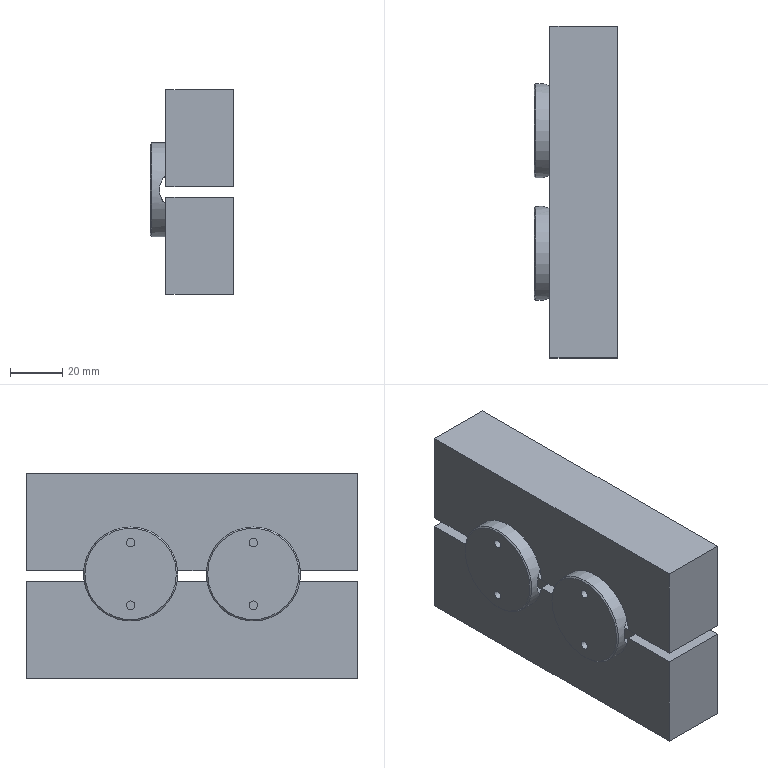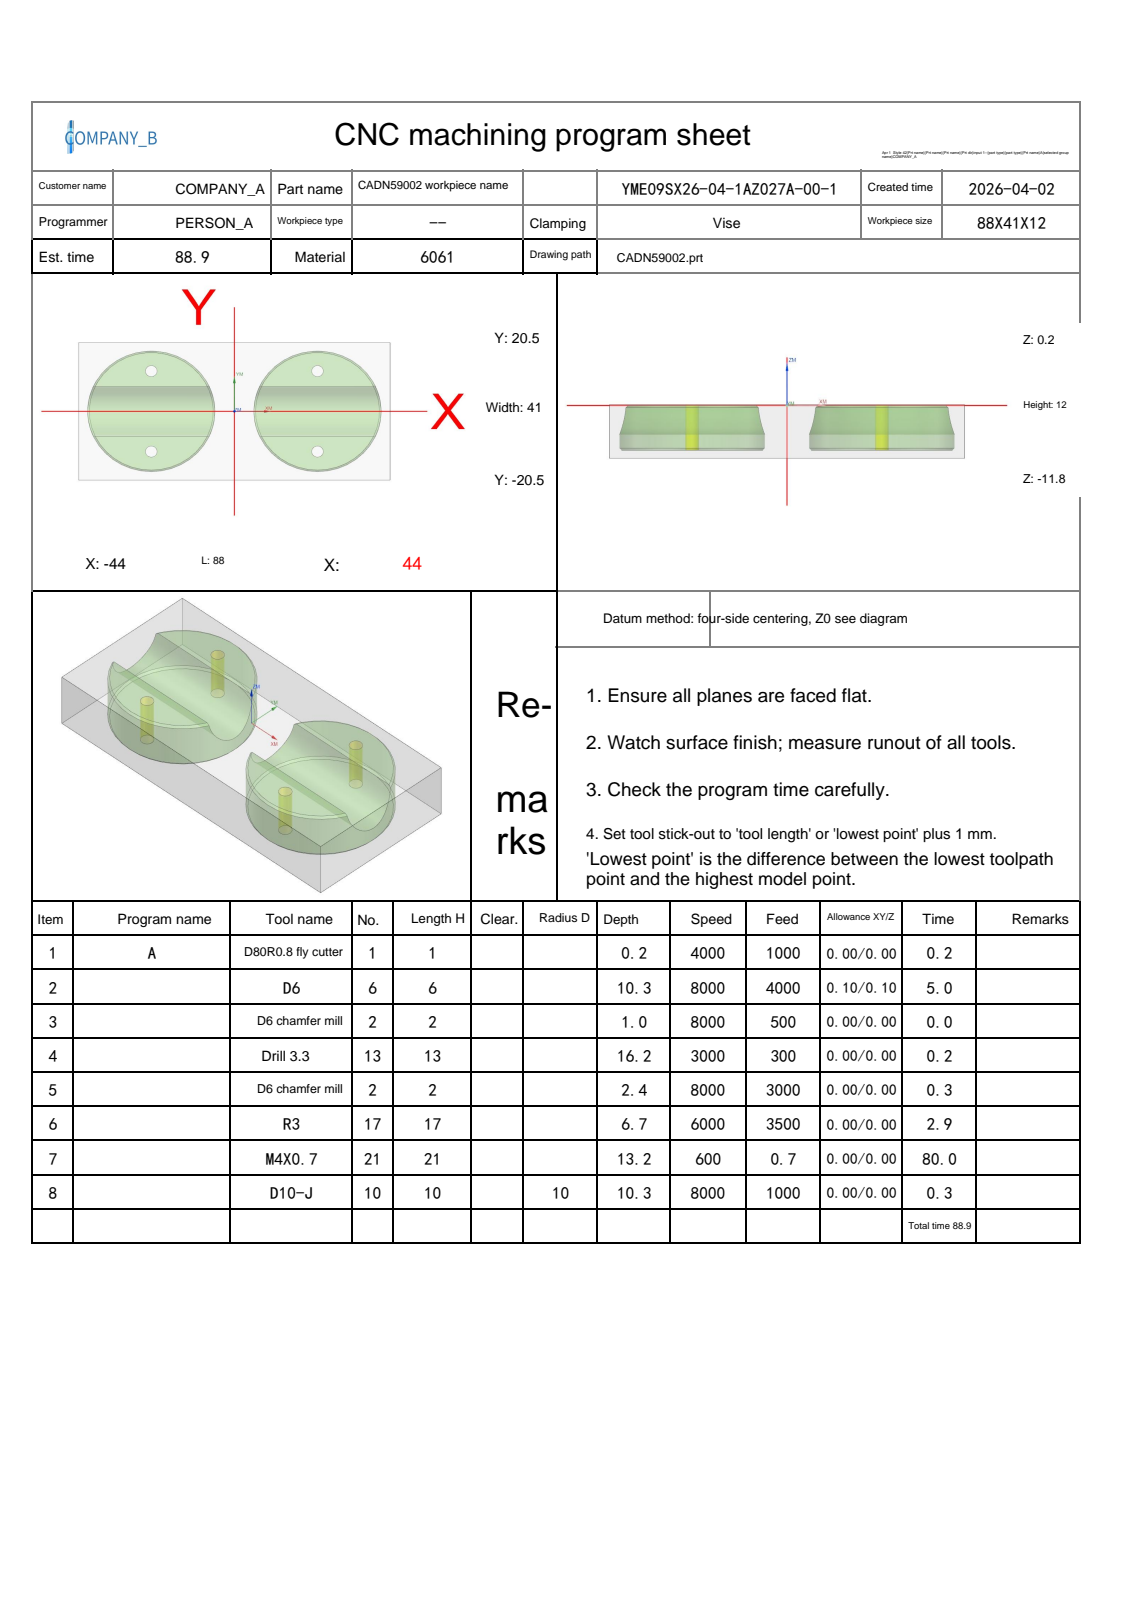NC program | NX | posted by the shop | part box 32 x 127 x 78.432 mm
Lines 34 to 1083 of 8369:
N2 T06 M06
(D6  D=6. R=0. H=06 ce=0.10 di=0.10)
G00 G90 G54 X-51.2 Y-4.2 M03 S8000
G43 H06 Z10.2
M08
Z.719
G01 Z-.481 F4000.
X-48.5
G03 X-44.3 Y0.0 I0.0 J4.2
G01 Y20.5
G02 X-44. Y20.8 I.3 J0.0
G01 X-39.372
G02 X-38.772 Y20.2 I0.0 J-.6
G01 X-38.78 Y20.1
X-39.137 Y17.99
G03 X-39.174 Y17.554 I2.581 J-.436
X-38.848 Y16.29 I2.618 J0.0
G02 X-38.774 Y16. I-.525 J-.29
X-38.95 Y15.575 I-.6 J0.0
G01 X-39.075 Y15.45
G02 X-39.5 Y15.274 I-.425 J.424
X-40.1 Y15.872 I0.0 J.6
G01 Y16.001
G02 X-39.83 Y16.501 I.6 J-.001
G03 X-39.56 Y17.002 I-.33 J.501
G01 X-39.565 Y17.081
X-39.967 Y20.121
X-39.972 Y20.2
G02 X-39.372 Y20.8 I.6 J0.0
G01 X-30.474
G02 X-23.5 Y21.938 I6.974 J-20.8
X-16.526 Y20.8 I0.0 J-21.938
G01 X16.526
G02 X23.5 Y21.938 I6.974 J-20.8
X30.474 Y20.8 I0.0 J-21.938
G01 X44.
G02 X44.3 Y20.5 I0.0 J-.3
G01 Y15.872
G02 X43.7 Y15.272 I-.6 J0.0
G01 X43.6 Y15.28
X41.49 Y15.637
G03 X41.054 Y15.674 I-.436 J-2.581
X39.79 Y15.348 I0.0 J-2.618
G02 X39.5 Y15.274 I-.29 J.525
X39.075 Y15.45 I0.0 J.6
G01 X38.95 Y15.575
G02 X38.774 Y16. I.424 J.425
X39.372 Y16.6 I.6 J0.0
G01 X39.501
G02 X40.001 Y16.33 I-.001 J-.6
G03 X40.502 Y16.06 I.501 J.33
G01 X40.581 Y16.065
X43.621 Y16.467
X43.7 Y16.472
G02 X44.3 Y15.872 I0.0 J-.6
G01 Y-20.5
G02 X44. Y-20.8 I-.3 J0.0
G01 X39.372
G02 X38.772 Y-20.2 I0.0 J.6
G01 X38.78 Y-20.1
X39.137 Y-17.99
G03 X39.174 Y-17.554 I-2.581 J.436
X38.848 Y-16.29 I-2.618 J0.0
G02 X38.774 Y-16. I.525 J.29
X38.95 Y-15.575 I.6 J0.0
G01 X39.075 Y-15.45
G02 X39.5 Y-15.274 I.425 J-.424
X40.1 Y-15.872 I0.0 J-.6
G01 Y-16.001
G02 X39.83 Y-16.501 I-.6 J.001
G03 X39.56 Y-17.002 I.33 J-.501
G01 X39.565 Y-17.081
X39.967 Y-20.121
X39.972 Y-20.2
G02 X39.372 Y-20.8 I-.6 J0.0
G01 X30.474
G02 X23.5 Y-21.938 I-6.974 J20.8
X16.526 Y-20.8 I0.0 J21.938
G01 X-16.526
G02 X-23.5 Y-21.938 I-6.974 J20.8
X-30.474 Y-20.8 I0.0 J21.938
G01 X-44.
G02 X-44.3 Y-20.5 I0.0 J.3
G01 Y-15.872
G02 X-43.7 Y-15.272 I.6 J0.0
G01 X-43.6 Y-15.28
X-41.49 Y-15.637
G03 X-41.054 Y-15.674 I.436 J2.581
X-39.79 Y-15.348 I0.0 J2.618
G02 X-39.5 Y-15.274 I.29 J-.525
X-39.075 Y-15.45 I0.0 J-.6
G01 X-38.95 Y-15.575
G02 X-38.774 Y-16. I-.424 J-.425
X-39.372 Y-16.6 I-.6 J0.0
G01 X-39.501
G02 X-40.001 Y-16.33 I.001 J.6
G03 X-40.502 Y-16.06 I-.501 J-.33
G01 X-40.581 Y-16.065
X-43.621 Y-16.467
X-43.7 Y-16.472
G02 X-44.3 Y-15.872 I0.0 J.6
G01 Y3.
G02 X-43.7 Y3.6 I.6 J0.0
G01 X-43.573 Y3.586
X-40.589 Y2.94
X-40.463 Y2.927
G03 X-39.982 Y3.168 I0.0 J.6
G02 X-39.501 Y3.41 I.482 J-.358
G01 X-7.068
G03 X-4.389 Y4.463 I-.001 J3.939
G02 X-4.185 Y4.587 I.408 J-.44
G01 X-1.896 Y5.416
G03 X-1.5 Y5.981 I-.204 J.564
G01 Y10.182
G02 X0.0 Y11.682 I1.5 J0.0
X1.5 Y10.182 I0.0 J-1.5
G01 Y4.372
G02 X0.0 Y2.872 I-1.5 J0.0
X-.984 Y3.24 I0.0 J1.5
G01 X-1.093 Y3.365
X-3.075 Y6.414
G02 X-3.171 Y6.741 I.503 J.327
G01 X-3.166 Y6.821
G03 X-3.13 Y7.349 I-3.903 J.528
X-3.474 Y8.958 I-3.939 J0.0
X-7.838 Y15.362 I-20.026 J-8.958
X-8.171 Y15.502 I-.334 J-.327
G01 X-8.33 Y15.474
X-8.55 Y15.395
G03 X-8.716 Y15.158 I.086 J-.237
G01 X-8.642 Y14.979
G02 X-4.241 Y8.615 I-14.858 J-14.979
X-3.97 Y7.349 I-2.828 J-1.266
X-7.068 Y4.25 I-3.099 J0.0
G01 X-39.932
G02 X-43.026 Y7.355 I.01 J3.104
X-42.751 Y8.634 I3.104 J0.0
X-23.5 Y21.098 I19.251 J-8.634
X-8.642 Y14.979 I0.0 J-21.098
G01 X-8.464 Y14.906
G03 X-8.226 Y15.074 I0.0 J.252
G01 X-8.095 Y15.448
X-8.081 Y15.528
X-8.123 Y15.663
G02 X-8.226 Y16. I.496 J.337
X-7.628 Y16.6 I.6 J0.0
G01 X7.628
G02 X8.226 Y16. I-.001 J-.6
X8.05 Y15.575 I-.6 J0.0
G03 X4.882 Y11.605 I15.45 J-15.575
G02 X4.373 Y11.322 I-.509 J.318
G01 X4.294 Y11.328
X.645 Y11.814
X.485 Y11.825
G03 X.08 Y11.755 I0.0 J-1.216
G01 X0.0 Y11.742
G02 X-.213 Y11.872 I0.0 J.24
G01 X-.305 Y12.05
X-.332 Y12.16
G02 X-.093 Y12.4 I.24 J0.0
G01 X.093
G02 X.331 Y12.181 I-.001 J-.24
G03 X.464 Y11.869 I.544 J.048
G01 X3.117 Y8.847
G02 X3.266 Y8.451 I-.451 J-.396
G01 X3.248 Y8.306
G03 X3.13 Y7.349 I3.821 J-.957
X7.068 Y3.41 I3.939 J0.0
G01 X39.206
G03 X39.628 Y3.677 I0.0 J.467
G01 X39.729 Y3.89
X39.753 Y3.998
G03 X39.501 Y4.25 I-.252 J0.0
G01 X7.068
G02 X3.97 Y7.349 I.001 J3.099
X4.241 Y8.615 I3.099 J0.0
X23.5 Y21.098 I19.259 J-8.615
X42.751 Y8.634 I0.0 J-21.098
X43.029 Y7.349 I-2.821 J-1.285
X39.929 Y4.249 I-3.1 J0.0
G01 X39.846 Y4.25
X39.501
G03 X39.249 Y3.998 I0.0 J-.252
G01 X39.274 Y3.89
X39.444 Y3.532
G03 X39.615 Y3.399 I.217 J.103
G02 X40.1 Y2.812 I-.115 J-.589
G01 Y.497
X40.088 Y.467
X40.059 Y.438
X40.039 Y.392
G02 X38.56 Y-1.071 I-1.5 J.037
G01 X4.521 Y-1.519
X4.501
G02 X3.001 Y-.019 I0.0 J1.5
X4.481 Y1.481 I1.5 J0.0
G01 X38.52 Y1.929
X38.54
G02 X40.038 Y.496 I0.0 J-1.5
G01 X40.051 Y.467
X40.08 Y.439
X40.1 Y.39
Y-2.812
G02 X39.501 Y-3.41 I-.6 J.001
G01 X7.068
G03 X3.13 Y-7.349 I.001 J-3.939
X3.166 Y-7.878 I3.939 J0.0
G01 X3.172 Y-7.958
G02 X3.032 Y-8.342 I-.6 J0.0
G01 X1.626 Y-10.03
G03 X1.491 Y-10.348 I.461 J-.384
G02 X0.0 Y-11.682 I-1.491 J.166
X-1.5 Y-10.182 I0.0 J1.5
G01 Y-4.372
G02 X0.0 Y-2.872 I1.5 J0.0
X1.5 Y-4.372 I0.0 J-1.5
G01 Y-8.648
G03 X1.846 Y-9.191 I.6 J0.0
G01 X3.921 Y-10.162
G02 X4.194 Y-10.42 I-.254 J-.543
G03 X7.838 Y-15.362 I19.306 J10.42
X8.171 Y-15.502 I.334 J.327
G01 X8.33 Y-15.474
X8.55 Y-15.395
G03 X8.716 Y-15.158 I-.086 J.237
G01 X8.642 Y-14.979
G02 X4.241 Y-8.615 I14.858 J14.979
X3.97 Y-7.349 I2.828 J1.266
X7.068 Y-4.25 I3.099 J0.0
G01 X39.932
G02 X43.026 Y-7.355 I-.01 J-3.104
X42.751 Y-8.634 I-3.104 J0.0
X23.5 Y-21.098 I-19.251 J8.634
X8.642 Y-14.979 I0.0 J21.098
G01 X8.464 Y-14.906
G03 X8.226 Y-15.074 I0.0 J-.252
G01 X8.095 Y-15.448
X8.081 Y-15.528
X8.123 Y-15.663
G02 X8.226 Y-16. I-.496 J-.337
X7.628 Y-16.6 I-.6 J0.0
G01 X-7.628
G02 X-8.226 Y-16. I.001 J.6
X-8.05 Y-15.575 I.6 J0.0
G03 X-4.882 Y-11.605 I-15.45 J15.575
G02 X-4.373 Y-11.322 I.509 J-.318
G01 X-4.294 Y-11.328
X-.645 Y-11.814
X-.485 Y-11.825
G03 X-.08 Y-11.755 I0.0 J1.216
G01 X0.0 Y-11.742
G02 X.213 Y-11.872 I0.0 J-.24
G01 X.305 Y-12.05
X.332 Y-12.16
G02 X.093 Y-12.4 I-.24 J0.0
G01 X-.093
G02 X-.331 Y-12.181 I.001 J.24
G03 X-.464 Y-11.869 I-.544 J-.048
G01 X-3.117 Y-8.847
G02 X-3.266 Y-8.451 I.451 J.396
G01 X-3.248 Y-8.306
G03 X-3.13 Y-7.349 I-3.821 J.957
X-3.722 Y-5.274 I-3.939 J0.0
G02 X-3.812 Y-4.958 I.51 J.316
G01 X-3.792 Y-4.806
X-2.752 Y-.828
X-2.732 Y-.676
G03 X-2.836 Y-.338 I-.6 J0.0
G02 X-2.941 Y0.0 I.496 J.338
X-2.667 Y.504 I.6 J0.0
G03 X-.484 Y2.566 I-4.402 J6.845
G02 X0.0 Y2.812 I.484 J-.354
X.484 Y2.566 I0.0 J-.6
G03 X2.667 Y.504 I6.585 J4.783
G02 X2.941 Y0.0 I-.326 J-.504
X2.667 Y-.504 I-.6 J0.0
G03 X.484 Y-2.566 I4.402 J-6.845
G02 X0.0 Y-2.812 I-.484 J.354
X-.484 Y-2.566 I0.0 J.6
G03 X-1.19 Y-1.721 I-6.585 J-4.783
X-1.623 Y-1.536 I-.433 J-.415
X-1.858 Y-1.584 I0.0 J-.6
G01 X-6.161 Y-3.413
G02 X-6.395 Y-3.461 I-.234 J.552
G01 X-6.484 Y-3.454
G03 X-7.068 Y-3.41 I-.585 J-3.895
G01 X-39.206
G03 X-39.628 Y-3.677 I0.0 J-.467
G01 X-39.729 Y-3.89
X-39.753 Y-3.998
G03 X-39.501 Y-4.25 I.252 J0.0
G01 X-7.068
G02 X-3.97 Y-7.349 I-.001 J-3.099
X-4.241 Y-8.615 I-3.099 J0.0
X-23.5 Y-21.098 I-19.259 J8.615
X-42.751 Y-8.634 I0.0 J21.098
X-43.029 Y-7.349 I2.821 J1.285
X-39.929 Y-4.249 I3.1 J0.0
G01 X-39.846 Y-4.25
X-39.501
G03 X-39.249 Y-3.998 I0.0 J.252
G01 X-39.274 Y-3.89
X-39.444 Y-3.532
G03 X-39.615 Y-3.399 I-.217 J-.103
G02 X-40.1 Y-2.812 I.115 J.589
G01 Y-.497
X-40.088 Y-.467
X-40.059 Y-.438
X-40.039 Y-.392
G02 X-38.56 Y1.071 I1.5 J-.037
G01 X-4.521 Y1.519
X-4.501
G02 X-3.001 Y.019 I0.0 J-1.5
X-4.481 Y-1.481 I-1.5 J0.0
G01 X-38.52 Y-1.929
X-38.54
G02 X-40.038 Y-.496 I0.0 J1.5
G01 X-40.051 Y-.467
X-40.08 Y-.439
X-40.1 Y-.39
Y0.0
Y2.834
G02 X-39.886 Y3.27 I.6 J-.024
G01 X-40.69 Y2.595 Z.569
G00 Z3.
G01 X-51.2 Y-4.2 F6000.
G00 Z.238
G01 Z-.962 F4000.
X-48.5
G03 X-44.3 Y0.0 I0.0 J4.2
G01 Y20.5
G02 X-44. Y20.8 I.3 J0.0
G01 X-39.375
G02 X-38.775 Y20.2 I0.0 J-.6
G01 X-38.783 Y20.1
X-39.14 Y17.988
G03 X-39.176 Y17.553 I2.577 J-.435
X-38.851 Y16.29 I2.614 J0.0
G02 X-38.776 Y16. I-.525 J-.29
X-38.952 Y15.575 I-.6 J0.0
G01 X-39.075 Y15.452
G02 X-39.5 Y15.276 I-.425 J.424
X-40.1 Y15.875 I0.0 J.6
G01 Y16.002
G02 X-39.83 Y16.501 I.6 J-.002
G03 X-39.56 Y17.002 I-.33 J.501
G01 X-39.565 Y17.081
X-39.969 Y20.121
X-39.975 Y20.2
G02 X-39.375 Y20.8 I.6 J0.0
G01 X-30.48
G02 X-23.5 Y21.94 I6.98 J-20.8
X-16.52 Y20.8 I0.0 J-21.94
G01 X16.52
G02 X23.5 Y21.94 I6.98 J-20.8
X30.48 Y20.8 I0.0 J-21.94
G01 X44.
G02 X44.3 Y20.5 I0.0 J-.3
G01 Y15.875
G02 X43.7 Y15.275 I-.6 J0.0
G01 X43.6 Y15.283
X41.488 Y15.64
G03 X41.053 Y15.676 I-.435 J-2.577
X39.79 Y15.351 I0.0 J-2.614
G02 X39.5 Y15.276 I-.29 J.525
X39.075 Y15.452 I0.0 J.6
G01 X38.952 Y15.575
G02 X38.776 Y16. I.424 J.425
X39.375 Y16.6 I.6 J0.0
G01 X39.502
G02 X40.001 Y16.33 I-.002 J-.6
G03 X40.502 Y16.06 I.501 J.33
G01 X40.581 Y16.065
X43.621 Y16.469
X43.7 Y16.475
G02 X44.3 Y15.875 I0.0 J-.6
G01 Y-20.5
G02 X44. Y-20.8 I-.3 J0.0
G01 X39.375
G02 X38.775 Y-20.2 I0.0 J.6
G01 X38.783 Y-20.1
X39.14 Y-17.988
G03 X39.176 Y-17.553 I-2.577 J.435
X38.851 Y-16.29 I-2.614 J0.0
G02 X38.776 Y-16. I.525 J.29
X38.952 Y-15.575 I.6 J0.0
G01 X39.075 Y-15.452
G02 X39.5 Y-15.276 I.425 J-.424
X40.1 Y-15.875 I0.0 J-.6
G01 Y-16.002
G02 X39.83 Y-16.501 I-.6 J.002
G03 X39.56 Y-17.002 I.33 J-.501
G01 X39.565 Y-17.081
X39.969 Y-20.121
X39.975 Y-20.2
G02 X39.375 Y-20.8 I-.6 J0.0
G01 X30.48
G02 X23.5 Y-21.94 I-6.98 J20.8
X16.52 Y-20.8 I0.0 J21.94
G01 X-16.52
G02 X-23.5 Y-21.94 I-6.98 J20.8
X-30.48 Y-20.8 I0.0 J21.94
G01 X-44.
G02 X-44.3 Y-20.5 I0.0 J.3
G01 Y-15.875
G02 X-43.7 Y-15.275 I.6 J0.0
G01 X-43.6 Y-15.283
X-41.488 Y-15.64
G03 X-41.053 Y-15.676 I.435 J2.577
X-39.79 Y-15.351 I0.0 J2.614
G02 X-39.5 Y-15.276 I.29 J-.525
X-39.075 Y-15.452 I0.0 J-.6
G01 X-38.952 Y-15.575
G02 X-38.776 Y-16. I-.424 J-.425
X-39.375 Y-16.6 I-.6 J0.0
G01 X-39.502
G02 X-40.001 Y-16.33 I.002 J.6
G03 X-40.502 Y-16.06 I-.501 J-.33
G01 X-40.581 Y-16.065
X-43.621 Y-16.469
X-43.7 Y-16.475
G02 X-44.3 Y-15.875 I0.0 J.6
G01 Y3.
G02 X-43.7 Y3.6 I.6 J0.0
G01 X-43.557 Y3.583
X-40.587 Y2.853
X-40.444 Y2.836
G03 X-39.972 Y3.065 I0.0 J.6
G02 X-39.502 Y3.295 I.472 J-.37
G01 X-7.08
X-7.009
G03 X-3.075 Y7.229 I0.0 J3.934
X-3.412 Y8.823 I-3.934 J0.0
X-7.835 Y15.362 I-20.088 J-8.823
X-8.169 Y15.502 I-.334 J-.327
G01 X-8.328 Y15.474
X-8.547 Y15.395
G03 X-8.714 Y15.158 I.086 J-.237
G01 X-8.639 Y14.979
G02 X-4.181 Y8.483 I-14.861 J-14.979
X-3.915 Y7.229 I-2.828 J-1.255
X-7.009 Y4.135 I-3.094 J0.0
G01 X-7.072
X-39.984
X-40.003
G02 X-43.089 Y7.221 I0.0 J3.086
X-42.819 Y8.483 I3.086 J0.0
X-23.5 Y21.1 I19.319 J-8.483
X-8.639 Y14.979 I0.0 J-21.1
G01 X-8.462 Y14.906
G03 X-8.224 Y15.074 I0.0 J.252
G01 X-8.092 Y15.448
X-8.079 Y15.528
X-8.12 Y15.663
G02 X-8.224 Y16. I.496 J.337
X-7.625 Y16.6 I.6 J0.0
G01 X7.625
G02 X8.224 Y16. I-.002 J-.6
X8.048 Y15.575 I-.6 J0.0
G03 X4.882 Y11.608 I15.452 J-15.575
G02 X4.373 Y11.326 I-.509 J.318
G01 X4.294 Y11.331
X.644 Y11.818
X.484 Y11.829
G03 X.08 Y11.759 I0.0 J-1.211
G01 X0.0 Y11.746
G02 X-.213 Y11.876 I0.0 J.24
G01 X-.303 Y12.05
X-.33 Y12.16
G02 X-.091 Y12.4 I.24 J0.0
G01 X.091
G02 X.329 Y12.181 I-.001 J-.24
G03 X.461 Y11.87 I.541 J.047
G01 X3.098 Y8.864
G02 X3.247 Y8.469 I-.451 J-.395
G01 X3.224 Y8.305
G03 X3.074 Y7.23 I3.786 J-1.075
X3.116 Y6.662 I3.935 J0.0
G01 X3.122 Y6.575
G02 X3.005 Y6.219 I-.6 J0.0
G01 X1.606 Y4.321
G03 X1.492 Y4.026 I.483 J-.356
G02 X0.0 Y2.677 I-1.492 J.151
X-1.5 Y4.177 I0.0 J1.5
G01 Y10.185
G02 X0.0 Y11.686 I1.5 J0.0
X1.5 Y10.186 I0.0 J-1.5
G01 Y5.785
G03 X1.903 Y5.219 I.6 J0.0
G01 X4.167 Y4.431
G02 X4.371 Y4.31 I-.197 J-.567
G03 X7.01 Y3.295 I2.638 J2.92
G01 X7.08
X39.206
G03 X39.628 Y3.562 I0.0 J.467
G01 X39.729 Y3.775
X39.754 Y3.883
G03 X39.502 Y4.135 I-.252 J0.0
G01 X7.072
X7.01
G02 X3.914 Y7.23 I0.0 J3.095
X4.209 Y8.549 I3.095 J0.0
X23.5 Y21.1 I19.291 J-8.549
X42.819 Y8.483 I0.0 J-21.1
X43.089 Y7.221 I-2.816 J-1.262
X40.003 Y4.135 I-3.086 J0.0
G01 X39.985
X39.502
G03 X39.25 Y3.883 I0.0 J-.252
G01 X39.274 Y3.775
X39.444 Y3.417
G03 X39.615 Y3.284 I.217 J.103
G02 X40.1 Y2.697 I-.115 J-.589
G01 Y.371
X40.088 Y.34
X40.059 Y.312
X40.039 Y.266
G02 X38.554 Y-1.191 I-1.499 J.042
G01 X4.281 Y-1.514
X4.267
G02 X2.767 Y-.014 I0.0 J1.5
X4.253 Y1.486 I1.5 J0.0
G01 X38.526 Y1.809
X38.54
G02 X40.039 Y.37 I0.0 J-1.5
G01 X40.051 Y.341
X40.08 Y.313
X40.1 Y.264
Y-2.697
G02 X39.502 Y-3.295 I-.6 J.002
G01 X7.016
X7.009
G03 X3.074 Y-7.23 I0.0 J-3.935
X3.445 Y-8.898 I3.935 J0.0
X7.835 Y-15.362 I20.055 J8.898
X8.169 Y-15.502 I.334 J.327
G01 X8.328 Y-15.474
X8.547 Y-15.395
G03 X8.714 Y-15.158 I-.086 J.237
G01 X8.639 Y-14.979
G02 X4.209 Y-8.549 I14.861 J14.979
X3.914 Y-7.23 I2.799 J1.319
X7.009 Y-4.135 I3.095 J0.0
G01 X7.015
X39.984
X40.003
G02 X43.089 Y-7.221 I0.0 J-3.086
X42.819 Y-8.483 I-3.086 J0.0
X23.5 Y-21.1 I-19.319 J8.483
X8.639 Y-14.979 I0.0 J21.1
G01 X8.462 Y-14.906
G03 X8.224 Y-15.074 I0.0 J-.252
G01 X8.092 Y-15.448
X8.079 Y-15.528
X8.12 Y-15.663
G02 X8.224 Y-16. I-.496 J-.337
X7.625 Y-16.6 I-.6 J0.0
G01 X-7.625
G02 X-8.224 Y-16. I.002 J.6
X-8.048 Y-15.575 I.6 J0.0
G03 X-4.882 Y-11.608 I-15.452 J15.575
G02 X-4.373 Y-11.326 I.509 J-.318
G01 X-4.294 Y-11.331
X-.644 Y-11.818
X-.484 Y-11.829
G03 X-.08 Y-11.759 I0.0 J1.211
G01 X0.0 Y-11.746
G02 X.213 Y-11.876 I0.0 J-.24
G01 X.303 Y-12.05
X.33 Y-12.16
G02 X.091 Y-12.4 I-.24 J0.0
G01 X-.091
G02 X-.324 Y-12.214 I.001 J.24
G03 X-.551 Y-11.885 I-.529 J-.122
G01 X-3.627 Y-9.831
G02 X-3.746 Y-9.608 I.149 J.223
G01 X-3.72 Y-9.492
X-3.698 Y-9.447
X-3.691 Y-9.377
X-3.622 Y-9.39
X-2.001 Y-9.118
G03 X-1.5 Y-8.526 I-.099 J.592
G01 Y-4.177
G02 X0.0 Y-2.677 I1.5 J0.0
X1.5 Y-4.177 I0.0 J-1.5
G01 Y-10.186
G02 X0.0 Y-11.686 I-1.5 J0.0
X-1.027 Y-11.279 I0.0 J1.5
G01 X-1.111 Y-11.18
X-3.039 Y-8.353
G02 X-3.143 Y-8.016 I.496 J.338
G01 X-3.134 Y-7.912
G03 X-3.074 Y-7.23 I-3.876 J.682
X-3.615 Y-5.239 I-3.935 J0.0
G02 X-3.698 Y-4.935 I.518 J.303
G01 X-3.674 Y-4.77
X-2.538 Y-.818
X-2.514 Y-.652
G03 X-2.611 Y-.326 I-.6 J0.0
G02 X-2.707 Y0.0 I.504 J.326
X-2.445 Y.495 I.6 J0.0
G03 X-.48 Y2.377 I-4.564 J6.733
G02 X0.0 Y2.617 I.48 J-.359
X.481 Y2.377 I0.0 J-.6
G03 X2.445 Y.496 I6.529 J4.853
G02 X2.707 Y0.0 I-.338 J-.496
X2.445 Y-.496 I-.6 J0.0
G03 X.48 Y-2.377 I4.563 J-6.734
G02 X0.0 Y-2.617 I-.48 J.359
X-.48 Y-2.377 I0.0 J.6
G03 X-.998 Y-1.749 I-6.529 J-4.853
X-1.441 Y-1.553 I-.443 J-.404
X-1.662 Y-1.595 I0.0 J-.6
G01 X-6.009 Y-3.32
G02 X-6.23 Y-3.362 I-.221 J.558
G01 X-6.332 Y-3.353
G03 X-7.01 Y-3.295 I-.677 J-3.877
G01 X-7.08
X-39.206
G03 X-39.628 Y-3.562 I0.0 J-.467
G01 X-39.729 Y-3.775
X-39.754 Y-3.883
G03 X-39.502 Y-4.135 I.252 J0.0
G01 X-7.072
X-7.01
G02 X-3.914 Y-7.23 I0.0 J-3.095
X-4.209 Y-8.549 I-3.095 J0.0
X-23.5 Y-21.1 I-19.291 J8.549
X-42.819 Y-8.483 I0.0 J21.1
X-43.089 Y-7.221 I2.816 J1.262
X-40.003 Y-4.135 I3.086 J0.0
G01 X-39.985
X-39.502
G03 X-39.25 Y-3.883 I0.0 J.252
G01 X-39.274 Y-3.775
X-39.444 Y-3.417
G03 X-39.615 Y-3.284 I-.217 J-.103
G02 X-40.1 Y-2.697 I.115 J.589
G01 Y.275
X-40.087 Y.305
X-40.058 Y.334
X-40.038 Y.379
G02 X-38.54 Y1.809 I1.498 J-.07
G01 X-38.526
X-4.253 Y1.486
G02 X-2.767 Y-.014 I-.014 J-1.5
X-4.267 Y-1.514 I-1.5 J0.0
G01 X-4.281
X-38.554 Y-1.191
G02 X-40.04 Y.276 I.014 J1.5
G01 X-40.052 Y.305
X-40.08 Y.333
X-40.1 Y.381
X-40.099 Y2.733
G02 X-39.874 Y3.164 I.599 J-.038
G01 X-40.695 Y2.509 Z.088
G00 Z2.519
G01 X-51.2 Y-4.2 F6000.
G00 Z-.243
G01 Z-1.443 F4000.
X-48.5
G03 X-44.3 Y0.0 I0.0 J4.2
G01 Y20.5
G02 X-44. Y20.8 I.3 J0.0
G01 X-39.374
G02 X-38.774 Y20.2 I0.0 J-.6
G01 X-38.783 Y20.1
X-39.14 Y17.988
G03 X-39.176 Y17.553 I2.577 J-.435
X-38.851 Y16.29 I2.614 J0.0
G02 X-38.776 Y16. I-.525 J-.29
X-38.952 Y15.575 I-.6 J0.0
G01 X-39.075 Y15.452
G02 X-39.5 Y15.276 I-.425 J.424
X-40.1 Y15.874 I0.0 J.6
G01 Y16.002
G02 X-39.83 Y16.501 I.6 J-.002
G03 X-39.56 Y17.002 I-.33 J.501
G01 X-39.566 Y17.081
X-39.969 Y20.121
X-39.974 Y20.2
G02 X-39.374 Y20.8 I.6 J0.0
G01 X-30.48
G02 X-23.5 Y21.94 I6.98 J-20.8
X-16.52 Y20.8 I0.0 J-21.94
G01 X16.52
G02 X23.5 Y21.94 I6.98 J-20.8
X30.48 Y20.8 I0.0 J-21.94
G01 X44.
G02 X44.3 Y20.5 I0.0 J-.3
G01 Y15.874
G02 X43.7 Y15.274 I-.6 J0.0
G01 X43.6 Y15.283
X41.488 Y15.64
G03 X41.053 Y15.676 I-.435 J-2.577
X39.79 Y15.351 I0.0 J-2.614
G02 X39.5 Y15.276 I-.29 J.525
X39.075 Y15.452 I0.0 J.6
G01 X38.952 Y15.575
G02 X38.776 Y16. I.424 J.425
X39.374 Y16.6 I.6 J0.0
G01 X39.502
G02 X40.001 Y16.33 I-.002 J-.6
G03 X40.502 Y16.06 I.501 J.33
G01 X40.581 Y16.066
X43.621 Y16.469
X43.7 Y16.474
G02 X44.3 Y15.874 I0.0 J-.6
G01 Y-20.5
G02 X44. Y-20.8 I-.3 J0.0
G01 X39.374
G02 X38.774 Y-20.2 I0.0 J.6
G01 X38.783 Y-20.1
X39.14 Y-17.988
G03 X39.176 Y-17.553 I-2.577 J.435
X38.851 Y-16.29 I-2.614 J0.0
G02 X38.776 Y-16. I.525 J.29
X38.952 Y-15.575 I.6 J0.0
G01 X39.075 Y-15.452
G02 X39.5 Y-15.276 I.425 J-.424
X40.1 Y-15.874 I0.0 J-.6
G01 Y-16.002
G02 X39.83 Y-16.501 I-.6 J.002
G03 X39.56 Y-17.002 I.33 J-.501
G01 X39.566 Y-17.081
X39.969 Y-20.121
X39.974 Y-20.2
G02 X39.374 Y-20.8 I-.6 J0.0
G01 X30.48
G02 X23.5 Y-21.94 I-6.98 J20.8
X16.52 Y-20.8 I0.0 J21.94
G01 X-16.52
G02 X-23.5 Y-21.94 I-6.98 J20.8
X-30.48 Y-20.8 I0.0 J21.94
G01 X-44.
G02 X-44.3 Y-20.5 I0.0 J.3
G01 Y-15.874
G02 X-43.7 Y-15.274 I.6 J0.0
G01 X-43.6 Y-15.283
X-41.488 Y-15.64
G03 X-41.053 Y-15.676 I.435 J2.577
X-39.79 Y-15.351 I0.0 J2.614
G02 X-39.5 Y-15.276 I.29 J-.525
X-39.075 Y-15.452 I0.0 J-.6
G01 X-38.952 Y-15.575
G02 X-38.776 Y-16. I-.424 J-.425
X-39.374 Y-16.6 I-.6 J0.0
G01 X-39.502
G02 X-40.001 Y-16.33 I.002 J.6
G03 X-40.502 Y-16.06 I-.501 J-.33
G01 X-40.581 Y-16.066
X-43.621 Y-16.469
X-43.7 Y-16.474
G02 X-44.3 Y-15.874 I0.0 J.6
G01 Y3.
G02 X-43.7 Y3.6 I.6 J0.0
G01 X-43.536 Y3.577
X-40.582 Y2.739
X-40.419 Y2.717
G03 X-39.96 Y2.931 I0.0 J.6
G02 X-39.502 Y3.145 I.46 J-.386
G01 X-6.608
G03 X-6.359 Y3.177 I0.0 J.978
G01 X-5.584 Y3.386
G03 X-4.357 Y4.118 I-1.377 J3.702
G02 X-4.15 Y4.237 I.395 J-.451
G01 X-1.918 Y4.975
G03 X-1.507 Y5.544 I-.188 J.57
G01 X-1.5 Y10.188
G02 X0.0 Y11.686 I1.5 J-.002
X1.5 Y10.186 I0.0 J-1.5
G01 Y10.183
X1.491 Y3.933
G02 X-.009 Y2.435 I-1.5 J.002
X-1.001 Y2.81 I0.0 J1.5
G01 X-1.115 Y2.946
X-2.99 Y5.999
G02 X-3.078 Y6.313 I.511 J.314
G01 X-3.07 Y6.415
G03 X-3.012 Y7.088 I-3.892 J.673
X-3.4 Y8.795 I-3.95 J0.0
X-7.836 Y15.362 I-20.1 J-8.795
X-8.169 Y15.502 I-.334 J-.327
G01 X-8.328 Y15.474
X-8.547 Y15.395
G03 X-8.714 Y15.158 I.086 J-.237
G01 X-8.639 Y14.979
G02 X-4.106 Y8.312 I-14.861 J-14.979
X-3.855 Y7.087 I-2.858 J-1.225
X-5.878 Y4.173 I-3.11 J0.0
G01 X-6.572 Y3.99
X-6.608 Y3.985
X-40.05
X-40.081
G02 X-43.159 Y7.063 I0.0 J3.078
X-42.895 Y8.31 I3.078 J0.0
X-23.5 Y21.1 I19.395 J-8.31
X-8.639 Y14.979 I0.0 J-21.1
G01 X-8.462 Y14.906
G03 X-8.224 Y15.074 I0.0 J.252
G01 X-8.092 Y15.449
X-8.079 Y15.528
X-8.12 Y15.663
G02 X-8.224 Y16. I.496 J.337
X-7.626 Y16.6 I.6 J0.0
G01 X7.626
G02 X8.224 Y16. I-.002 J-.6
X8.048 Y15.575 I-.6 J0.0
G03 X4.882 Y11.608 I15.452 J-15.575
G02 X4.373 Y11.326 I-.509 J.318
G01 X4.294 Y11.331
X.644 Y11.818
X.484 Y11.829
G03 X.08 Y11.759 I0.0 J-1.21
G01 X0.0 Y11.746
G02 X-.213 Y11.875 I0.0 J.24
G01 X-.303 Y12.05
X-.33 Y12.16
G02 X-.091 Y12.4 I.24 J0.0
G01 X.091
G02 X.329 Y12.181 I-.001 J-.24
G03 X.461 Y11.87 I.541 J.047
G01 X3.081 Y8.88
G02 X3.23 Y8.485 I-.451 J-.395
G01 X3.2 Y8.297
G03 X3.002 Y7.068 I3.726 J-1.229
X6.926 Y3.144 I3.924 J0.0
G01 X7.021 Y3.145
X39.206
G03 X39.628 Y3.412 I0.0 J.467
G01 X39.729 Y3.625
X39.754 Y3.733
G03 X39.502 Y3.985 I-.252 J0.0
G01 X7.01
X6.929 Y3.984
G02 X3.843 Y7.07 I0.0 J3.086
X4.142 Y8.396 I3.086 J0.0
G01 X4.209 Y8.549
G02 X23.5 Y21.1 I19.291 J-8.549
X42.895 Y8.31 I0.0 J-21.1
X43.151 Y7.077 I-2.837 J-1.232
X40.058 Y3.985 I-3.093 J0.0
G01 X39.997
X39.502
G03 X39.25 Y3.733 I0.0 J-.252
G01 X39.274 Y3.625
X39.444 Y3.267
G03 X39.615 Y3.134 I.217 J.103
G02 X40.1 Y2.547 I-.115 J-.589
G01 Y.207
X40.088 Y.177
X40.059 Y.148
X40.039 Y.103
G02 X38.547 Y-1.348 I-1.499 J.049
G01 X3.987 Y-1.514
X3.98
G02 X2.48 Y-.014 I0.0 J1.5
X3.973 Y1.486 I1.5 J0.0
G01 X38.533 Y1.652
X38.54
G02 X40.039 Y.206 I0.0 J-1.5
G01 X40.052 Y.177
X40.08 Y.149
X40.1 Y.101
Y-2.547
G02 X39.502 Y-3.145 I-.6 J.002
G01 X6.608
G03 X6.358 Y-3.178 I0.0 J-.978
G01 X5.587 Y-3.385
G03 X3.011 Y-7.082 I1.364 J-3.697
X3.093 Y-7.883 I3.94 J0.0
G01 X3.105 Y-8.005
G02 X2.97 Y-8.384 I-.6 J0.0
G01 X1.622 Y-10.038
G03 X1.491 Y-10.351 I.465 J-.379
G02 X0.0 Y-11.686 I-1.491 J.165
X-1.5 Y-10.186 I0.0 J1.5
G01 Y-10.185
X-1.494 Y-3.933
G02 X.006 Y-2.434 I1.5 J-.001
X1.506 Y-3.934 I0.0 J-1.5
G01 Y-3.936
X1.502 Y-8.653
G03 X1.848 Y-9.197 I.6 J0.0
G01 X3.922 Y-10.167
G02 X4.195 Y-10.425 I-.254 J-.543
G03 X7.836 Y-15.362 I19.305 J10.425
X8.169 Y-15.502 I.334 J.327
G01 X8.328 Y-15.474
X8.547 Y-15.395
G03 X8.714 Y-15.158 I-.086 J.237
G01 X8.639 Y-14.979
G02 X4.209 Y-8.549 I14.861 J14.979
X4.105 Y-8.31 I2.785 J1.356
X3.851 Y-7.081 I2.846 J1.228
X5.878 Y-4.173 I3.1 J0.0
G01 X6.572 Y-3.99
X6.608 Y-3.985
X40.05
X40.081
G02 X43.159 Y-7.063 I0.0 J-3.078
X42.895 Y-8.31 I-3.078 J0.0
G01 X42.819 Y-8.483
G02 X23.5 Y-21.1 I-19.319 J8.483
X8.639 Y-14.979 I0.0 J21.1
G01 X8.462 Y-14.906
G03 X8.224 Y-15.074 I0.0 J-.252
G01 X8.092 Y-15.448
X8.079 Y-15.528
X8.12 Y-15.663
G02 X8.224 Y-16. I-.496 J-.337
X7.626 Y-16.6 I-.6 J0.0
G01 X-7.626
G02 X-8.224 Y-16. I.002 J.6
X-8.048 Y-15.575 I.6 J0.0
G03 X-6.614 Y-14.009 I-15.452 J15.575
X-4.882 Y-11.608 I-16.884 J14.01
G02 X-4.373 Y-11.326 I.509 J-.318
G01 X-4.294 Y-11.331
X-.643 Y-11.819
X-.483 Y-11.829
G03 X-.08 Y-11.76 I0.0 J1.21
G01 X0.0 Y-11.746
G02 X.214 Y-11.876 I0.0 J-.24
G01 X.303 Y-12.05
X.33 Y-12.16
G02 X.091 Y-12.4 I-.24 J0.0
G01 X-.09
G02 X-.328 Y-12.181 I.001 J.24
G03 X-.461 Y-11.87 I-.54 J-.047
G01 X-3.082 Y-8.879
G02 X-3.231 Y-8.484 I.451 J.395
G01 X-3.201 Y-8.296
G03 X-3.004 Y-7.068 I-3.727 J1.228
X-3.484 Y-5.186 I-3.924 J0.0
G02 X-3.558 Y-4.899 I.527 J.288
G01 X-3.529 Y-4.716
X-2.277 Y-.798
X-2.249 Y-.616
G03 X-2.336 Y-.305 I-.6 J0.0
G02 X-2.423 Y.006 I.513 J.311
X-2.177 Y.491 I.6 J0.0
G03 X-.485 Y2.141 I-4.785 J6.597
G02 X-.009 Y2.375 I.476 J-.366
X.467 Y2.141 I0.0 J-.6
G03 X2.173 Y.48 I6.459 J4.927
G02 X2.42 Y-.006 I-.353 J-.485
X2.174 Y-.49 I-.6 J0.0
G03 X.482 Y-2.14 I4.777 J-6.591
G02 X.007 Y-2.374 I-.476 J.366
X-.469 Y-2.14 I0.0 J.6
G03 X-.765 Y-1.774 I-6.459 J-4.928
X-1.22 Y-1.565 I-.455 J-.391
X-1.425 Y-1.601 I0.0 J-.6
G01 X-5.82 Y-3.199
G02 X-6.025 Y-3.235 I-.205 J.564
G01 X-6.144 Y-3.223
G03 X-6.928 Y-3.144 I-.783 J-3.845
G01 X-7.021 Y-3.145
X-39.206
G03 X-39.628 Y-3.412 I0.0 J-.467
G01 X-39.729 Y-3.625
X-39.754 Y-3.733
G03 X-39.502 Y-3.985 I.252 J0.0
G01 X-7.01
X-6.928 Y-3.984
G02 X-3.844 Y-7.068 I0.0 J-3.084
X-4.104 Y-8.31 I-3.084 J0.0
G01 X-4.144 Y-8.401
X-4.209 Y-8.549
G02 X-23.5 Y-21.1 I-19.291 J8.549
X-42.901 Y-8.295 I0.0 J21.1
X-43.15 Y-7.079 I2.845 J1.216
X-40.057 Y-3.985 I3.094 J0.0
G01 X-39.502
G03 X-39.25 Y-3.733 I0.0 J.252
G01 X-39.274 Y-3.625
X-39.444 Y-3.267
G03 X-39.615 Y-3.134 I-.217 J-.103
G02 X-40.1 Y-2.547 I.115 J.589
G01 Y-.207
X-40.088 Y-.177
X-40.059 Y-.148
X-40.039 Y-.103
G02 X-38.547 Y1.348 I1.499 J-.049
G01 X-3.99 Y1.513
X-3.983
G02 X-2.483 Y.013 I0.0 J-1.5
X-3.975 Y-1.487 I-1.5 J0.0
G01 X-38.533 Y-1.652
X-38.54
G02 X-40.039 Y-.206 I0.0 J1.5
G01 X-40.052 Y-.177
X-40.08 Y-.149
X-40.1 Y-.101
Y0.0
X-40.097 Y2.602
G02 X-39.86 Y3.025 I.597 J-.057
G01 X-40.7 Y2.396 Z-.393
G00 Z2.038
G01 X-51.2 Y-4.2 F6000.
G00 Z-.724
G01 Z-1.924 F4000.
X-48.5
G03 X-44.3 Y0.0 I0.0 J4.2
G01 Y20.5
G02 X-44. Y20.8 I.3 J0.0
G01 X-39.374
G02 X-38.774 Y20.2 I0.0 J-.6
G01 X-38.783 Y20.1
X-39.14 Y17.988
G03 X-39.176 Y17.553 I2.577 J-.435
X-38.851 Y16.29 I2.613 J0.0
G02 X-38.776 Y16. I-.525 J-.29
X-38.952 Y15.575 I-.6 J0.0
G01 X-39.075 Y15.452
G02 X-39.5 Y15.276 I-.425 J.424
X-40.1 Y15.874 I0.0 J.6
G01 Y16.002
G02 X-39.83 Y16.501 I.6 J-.002
G03 X-39.56 Y17.002 I-.33 J.501
G01 X-39.566 Y17.081
X-39.969 Y20.121
X-39.974 Y20.2
G02 X-39.374 Y20.8 I.6 J0.0
G01 X-30.48
G02 X-23.5 Y21.94 I6.98 J-20.8
X-16.52 Y20.8 I0.0 J-21.94
G01 X16.52
G02 X23.5 Y21.94 I6.98 J-20.8
X30.48 Y20.8 I0.0 J-21.94
G01 X44.
G02 X44.3 Y20.5 I0.0 J-.3
G01 Y15.874
G02 X43.7 Y15.274 I-.6 J0.0
G01 X43.6 Y15.283
X41.488 Y15.64
G03 X41.053 Y15.676 I-.435 J-2.577
X39.79 Y15.351 I0.0 J-2.613
G02 X39.5 Y15.276 I-.29 J.525
X39.075 Y15.452 I0.0 J.6
G01 X38.952 Y15.575
G02 X38.776 Y16. I.424 J.425
X39.374 Y16.6 I.6 J0.0
G01 X39.502
G02 X40.001 Y16.33 I-.002 J-.6
G03 X40.502 Y16.06 I.501 J.33
G01 X40.581 Y16.066
X43.621 Y16.469
X43.7 Y16.474